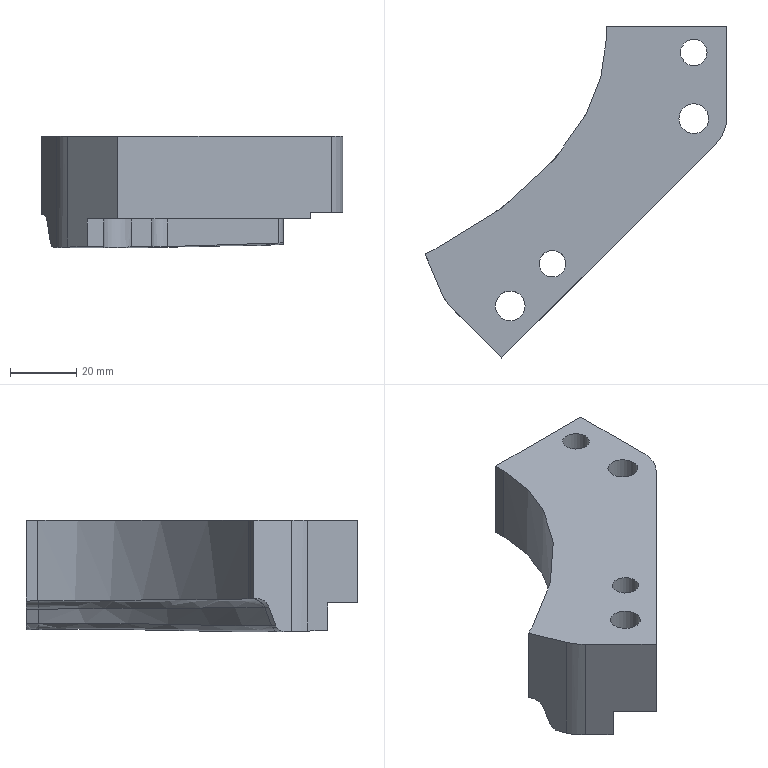Part | STEP file | 813_id1614_x_t | 1 solid | 49 faces | box 91.216 x 100.295 x 33.785 mm | volume 99685 mm3 | spline 20 | plane 18 | cylinder 11 | commonest cylinder face diameters 10 x3 8 x2 9 x2 14 x2 24 x1 30 x1